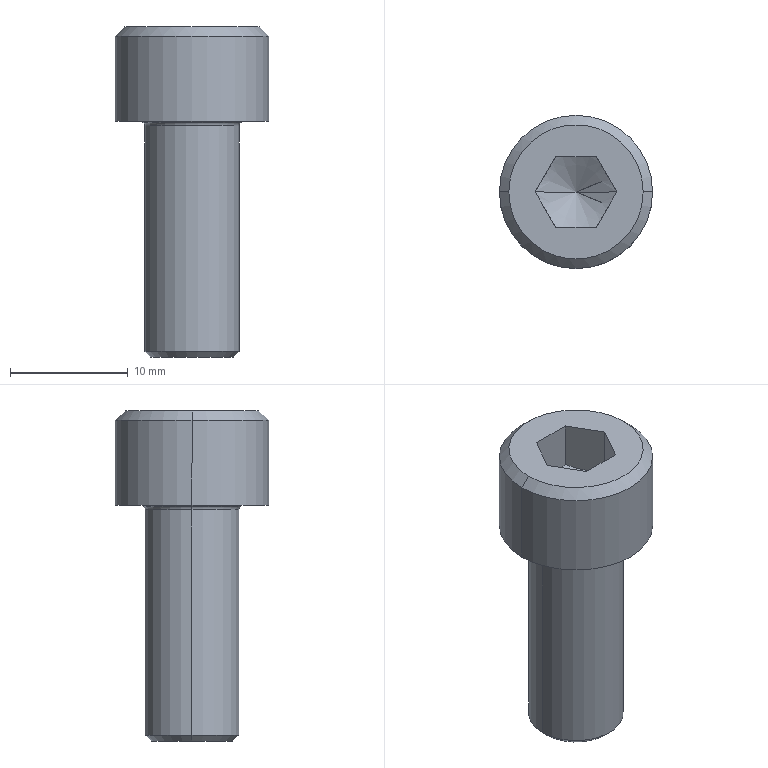Part | Creo | 1 solid | 23 faces | box 13 x 13 x 28 mm | volume 1903 mm3 | plane 9 | cone 6 | cylinder 4 | torus 4 | commonest cylinder face diameters 8 x2 13 x2
STEP:
#1=CARTESIAN_POINT('',(-151.536,-0.004699,-50.5));
#2=VERTEX_POINT('',#1);
#3=CARTESIAN_POINT('',(-153.268,2.995,-50.5));
#4=VERTEX_POINT('',#3);
#5=CARTESIAN_POINT('',(-151.536,-0.004699,-50.5));
#6=CARTESIAN_POINT('',(-151.583,0.07635,-50.527));
#7=CARTESIAN_POINT('',(-151.675,0.236,-50.577));
#8=CARTESIAN_POINT('',(-151.808,0.4663,-50.639));
#9=CARTESIAN_POINT('',(-151.939,0.6927,-50.689));
#10=CARTESIAN_POINT('',(-152.069,0.9189,-50.728));
#11=CARTESIAN_POINT('',(-152.201,1.148,-50.755));
#12=CARTESIAN_POINT('',(-152.335,1.379,-50.769));
#13=CARTESIAN_POINT('',(-152.469,1.612,-50.769));
#14=CARTESIAN_POINT('',(-152.602,1.843,-50.755));
#15=CARTESIAN_POINT('',(-152.735,2.072,-50.728));
#16=CARTESIAN_POINT('',(-152.865,2.298,-50.689));
#17=CARTESIAN_POINT('',(-152.996,2.524,-50.639));
#18=CARTESIAN_POINT('',(-153.129,2.755,-50.577));
#19=CARTESIAN_POINT('',(-153.221,2.914,-50.527));
#20=CARTESIAN_POINT('',(-153.268,2.995,-50.5));
#21=B_SPLINE_CURVE_WITH_KNOTS('',3,(#5,#6,#7,#8,#9,#10,#11,#12,#13,#14,#15,#16,#17,#18,#19,#20),.UNSPECIFIED.,.F.,.F.,(4,1,1,1,1,1,1,1,1,1,1,1,1,4),(0.,0.07692,0.1538,0.2308,0.3077,0.3846,0.4615,0.5385,0.6154,0.6923,0.7692,0.8462,0.9231,1.),.UNSPECIFIED.);
#22=EDGE_CURVE('',#2,#4,#21,.T.);
#23=ORIENTED_EDGE('',*,*,#22,.F.);
#24=CARTESIAN_POINT('',(-155.,-0.004699,-52.5));
#25=VERTEX_POINT('',#24);
#26=CARTESIAN_POINT('',(-155.,-0.004699,-52.5));
#27=DIRECTION('',(0.866,0.,0.5));
#28=VECTOR('',#27,4.);
#29=LINE('',#26,#28);
#30=EDGE_CURVE('',#25,#2,#29,.T.);
#31=ORIENTED_EDGE('',*,*,#30,.F.);
#32=CARTESIAN_POINT('',(-158.464,-0.004699,-50.5));
#33=VERTEX_POINT('',#32);
#34=CARTESIAN_POINT('',(-155.,-0.004699,-52.5));
#35=DIRECTION('',(-0.866,0.,0.5));
#36=VECTOR('',#35,4.);
#37=LINE('',#34,#36);
#38=EDGE_CURVE('',#25,#33,#37,.T.);
#39=ORIENTED_EDGE('',*,*,#38,.T.);
#40=CARTESIAN_POINT('',(-156.732,2.995,-50.5));
#41=VERTEX_POINT('',#40);
#42=CARTESIAN_POINT('',(-156.732,2.995,-50.5));
#43=CARTESIAN_POINT('',(-156.779,2.914,-50.527));
#44=CARTESIAN_POINT('',(-156.871,2.755,-50.577));
#45=CARTESIAN_POINT('',(-157.004,2.524,-50.639));
#46=CARTESIAN_POINT('',(-157.135,2.298,-50.689));
#47=CARTESIAN_POINT('',(-157.265,2.072,-50.728));
#48=CARTESIAN_POINT('',(-157.398,1.843,-50.755));
#49=CARTESIAN_POINT('',(-157.531,1.612,-50.769));
#50=CARTESIAN_POINT('',(-157.665,1.379,-50.769));
#51=CARTESIAN_POINT('',(-157.799,1.148,-50.755));
#52=CARTESIAN_POINT('',(-157.931,0.9189,-50.728));
#53=CARTESIAN_POINT('',(-158.061,0.6927,-50.689));
#54=CARTESIAN_POINT('',(-158.192,0.4663,-50.639));
#55=CARTESIAN_POINT('',(-158.325,0.236,-50.577));
#56=CARTESIAN_POINT('',(-158.417,0.07635,-50.527));
#57=CARTESIAN_POINT('',(-158.464,-0.004699,-50.5));
#58=B_SPLINE_CURVE_WITH_KNOTS('',3,(#42,#43,#44,#45,#46,#47,#48,#49,#50,#51,#52,#53,#54,#55,#56,#57),.UNSPECIFIED.,.F.,.F.,(4,1,1,1,1,1,1,1,1,1,1,1,1,4),(0.,0.07692,0.1538,0.2308,0.3077,0.3846,0.4615,0.5385,0.6154,0.6923,0.7692,0.8462,0.9231,1.),.UNSPECIFIED.);
#59=EDGE_CURVE('',#41,#33,#58,.T.);
#60=ORIENTED_EDGE('',*,*,#59,.F.);
#61=CARTESIAN_POINT('',(-153.268,2.995,-50.5));
#62=CARTESIAN_POINT('',(-153.361,2.995,-50.527));
#63=CARTESIAN_POINT('',(-153.545,2.995,-50.577));
#64=CARTESIAN_POINT('',(-153.811,2.995,-50.639));
#65=CARTESIAN_POINT('',(-154.072,2.995,-50.689));
#66=CARTESIAN_POINT('',(-154.333,2.995,-50.728));
#67=CARTESIAN_POINT('',(-154.598,2.995,-50.755));
#68=CARTESIAN_POINT('',(-154.865,2.995,-50.769));
#69=CARTESIAN_POINT('',(-155.135,2.995,-50.769));
#70=CARTESIAN_POINT('',(-155.402,2.995,-50.755));
#71=CARTESIAN_POINT('',(-155.667,2.995,-50.728));
#72=CARTESIAN_POINT('',(-155.928,2.995,-50.689));
#73=CARTESIAN_POINT('',(-156.189,2.995,-50.639));
#74=CARTESIAN_POINT('',(-156.455,2.995,-50.577));
#75=CARTESIAN_POINT('',(-156.639,2.995,-50.527));
#76=CARTESIAN_POINT('',(-156.732,2.995,-50.5));
#77=B_SPLINE_CURVE_WITH_KNOTS('',3,(#61,#62,#63,#64,#65,#66,#67,#68,#69,#70,#71,#72,#73,#74,#75,#76),.UNSPECIFIED.,.F.,.F.,(4,1,1,1,1,1,1,1,1,1,1,1,1,4),(0.,0.07692,0.1538,0.2308,0.3077,0.3846,0.4615,0.5385,0.6154,0.6923,0.7692,0.8462,0.9231,1.),.UNSPECIFIED.);
#78=EDGE_CURVE('',#4,#41,#77,.T.);
#79=ORIENTED_EDGE('',*,*,#78,.F.);
#80=EDGE_LOOP('',(#23,#31,#39,#60,#79));
#81=FACE_OUTER_BOUND('',#80,.F.);
#82=CARTESIAN_POINT('',(-155.,-0.004699,-51.48));
#83=DIRECTION('',(0.,0.,1.));
#84=DIRECTION('',(1.,0.,0.));
#85=AXIS2_PLACEMENT_3D('',#82,#83,#84);
#86=CONICAL_SURFACE('',#85,1.767,60.);
#87=ADVANCED_FACE('',(#81),#86,.F.);
#88=CARTESIAN_POINT('',(-153.268,2.995,-46.5));
#89=VERTEX_POINT('',#88);
#90=CARTESIAN_POINT('',(-151.536,-0.004699,-46.5));
#91=VERTEX_POINT('',#90);
#92=CARTESIAN_POINT('',(-153.268,2.995,-46.5));
#93=DIRECTION('',(0.5,-0.866,0.));
#94=VECTOR('',#93,3.464);
#95=LINE('',#92,#94);
#96=EDGE_CURVE('',#89,#91,#95,.T.);
#97=ORIENTED_EDGE('',*,*,#96,.T.);
#98=CARTESIAN_POINT('',(-151.536,-0.004699,-46.5));
#99=DIRECTION('',(0.,0.,-1.));
#100=VECTOR('',#99,4.);
#101=LINE('',#98,#100);
#102=EDGE_CURVE('',#91,#2,#101,.T.);
#103=ORIENTED_EDGE('',*,*,#102,.T.);
#104=ORIENTED_EDGE('',*,*,#22,.T.);
#105=CARTESIAN_POINT('',(-153.268,2.995,-46.5));
#106=DIRECTION('',(0.,0.,-1.));
#107=VECTOR('',#106,4.);
#108=LINE('',#105,#107);
#109=EDGE_CURVE('',#89,#4,#108,.T.);
#110=ORIENTED_EDGE('',*,*,#109,.F.);
#111=EDGE_LOOP('',(#97,#103,#104,#110));
#112=FACE_OUTER_BOUND('',#111,.F.);
#113=CARTESIAN_POINT('',(-153.268,2.995,-50.5));
#114=DIRECTION('',(-0.866,-0.5,0.));
#115=DIRECTION('',(0.5,-0.866,0.));
#116=AXIS2_PLACEMENT_3D('',#113,#114,#115);
#117=PLANE('',#116);
#118=ADVANCED_FACE('',(#112),#117,.T.);
#119=CARTESIAN_POINT('',(-149.3,-0.004699,-46.5));
#120=VERTEX_POINT('',#119);
#121=CARTESIAN_POINT('',(-160.7,-0.004699,-46.5));
#122=VERTEX_POINT('',#121);
#123=CARTESIAN_POINT('',(-155.,-0.004699,-46.5));
#124=DIRECTION('',(0.,0.,1.));
#125=DIRECTION('',(1.,0.,0.));
#126=AXIS2_PLACEMENT_3D('',#123,#124,#125);
#127=CIRCLE('',#126,5.7);
#128=EDGE_CURVE('',#120,#122,#127,.T.);
#129=ORIENTED_EDGE('',*,*,#128,.F.);
#130=CARTESIAN_POINT('',(-155.,-0.004699,-46.5));
#131=DIRECTION('',(0.,0.,1.));
#132=DIRECTION('',(-1.,0.,0.));
#133=AXIS2_PLACEMENT_3D('',#130,#131,#132);
#134=CIRCLE('',#133,5.7);
#135=EDGE_CURVE('',#122,#120,#134,.T.);
#136=ORIENTED_EDGE('',*,*,#135,.F.);
#137=EDGE_LOOP('',(#129,#136));
#138=FACE_OUTER_BOUND('',#137,.F.);
#139=CARTESIAN_POINT('',(-153.268,-3.005,-46.5));
#140=VERTEX_POINT('',#139);
#141=CARTESIAN_POINT('',(-151.536,-0.004699,-46.5));
#142=DIRECTION('',(-0.5,-0.866,0.));
#143=VECTOR('',#142,3.464);
#144=LINE('',#141,#143);
#145=EDGE_CURVE('',#91,#140,#144,.T.);
#146=ORIENTED_EDGE('',*,*,#145,.F.);
#147=ORIENTED_EDGE('',*,*,#96,.F.);
#148=CARTESIAN_POINT('',(-156.732,2.995,-46.5));
#149=VERTEX_POINT('',#148);
#150=CARTESIAN_POINT('',(-153.268,2.995,-46.5));
#151=DIRECTION('',(-1.,0.,0.));
#152=VECTOR('',#151,3.464);
#153=LINE('',#150,#152);
#154=EDGE_CURVE('',#89,#149,#153,.T.);
#155=ORIENTED_EDGE('',*,*,#154,.T.);
#156=CARTESIAN_POINT('',(-158.464,-0.004699,-46.5));
#157=VERTEX_POINT('',#156);
#158=CARTESIAN_POINT('',(-158.464,-0.004699,-46.5));
#159=DIRECTION('',(0.5,0.866,0.));
#160=VECTOR('',#159,3.464);
#161=LINE('',#158,#160);
#162=EDGE_CURVE('',#157,#149,#161,.T.);
#163=ORIENTED_EDGE('',*,*,#162,.F.);
#164=CARTESIAN_POINT('',(-156.732,-3.005,-46.5));
#165=VERTEX_POINT('',#164);
#166=CARTESIAN_POINT('',(-156.732,-3.005,-46.5));
#167=DIRECTION('',(-0.5,0.866,0.));
#168=VECTOR('',#167,3.464);
#169=LINE('',#166,#168);
#170=EDGE_CURVE('',#165,#157,#169,.T.);
#171=ORIENTED_EDGE('',*,*,#170,.F.);
#172=CARTESIAN_POINT('',(-156.732,-3.005,-46.5));
#173=DIRECTION('',(1.,0.,0.));
#174=VECTOR('',#173,3.464);
#175=LINE('',#172,#174);
#176=EDGE_CURVE('',#165,#140,#175,.T.);
#177=ORIENTED_EDGE('',*,*,#176,.T.);
#178=EDGE_LOOP('',(#146,#147,#155,#163,#171,#177));
#179=FACE_BOUND('',#178,.F.);
#180=CARTESIAN_POINT('',(-155.,-0.004699,-46.5));
#181=DIRECTION('',(0.,0.,1.));
#182=DIRECTION('',(1.,0.,0.));
#183=AXIS2_PLACEMENT_3D('',#180,#181,#182);
#184=PLANE('',#183);
#185=ADVANCED_FACE('',(#138,#179),#184,.T.);
#186=CARTESIAN_POINT('',(-148.5,-0.004699,-47.3));
#187=VERTEX_POINT('',#186);
#188=CARTESIAN_POINT('',(-161.5,-0.004699,-47.3));
#189=VERTEX_POINT('',#188);
#190=CARTESIAN_POINT('',(-155.,-0.004699,-47.3));
#191=DIRECTION('',(0.,0.,1.));
#192=DIRECTION('',(1.,0.,0.));
#193=AXIS2_PLACEMENT_3D('',#190,#191,#192);
#194=CIRCLE('',#193,6.5);
#195=EDGE_CURVE('',#187,#189,#194,.T.);
#196=ORIENTED_EDGE('',*,*,#195,.F.);
#197=CARTESIAN_POINT('',(-149.3,-0.004699,-46.5));
#198=DIRECTION('',(0.7071,0.,-0.7071));
#199=VECTOR('',#198,1.131);
#200=LINE('',#197,#199);
#201=EDGE_CURVE('',#120,#187,#200,.T.);
#202=ORIENTED_EDGE('',*,*,#201,.F.);
#203=ORIENTED_EDGE('',*,*,#128,.T.);
#204=CARTESIAN_POINT('',(-160.7,-0.004699,-46.5));
#205=DIRECTION('',(-0.7071,0.,-0.7071));
#206=VECTOR('',#205,1.131);
#207=LINE('',#204,#206);
#208=EDGE_CURVE('',#122,#189,#207,.T.);
#209=ORIENTED_EDGE('',*,*,#208,.T.);
#210=EDGE_LOOP('',(#196,#202,#203,#209));
#211=FACE_OUTER_BOUND('',#210,.F.);
#212=CARTESIAN_POINT('',(-155.,-0.004699,-46.9));
#213=DIRECTION('',(0.,0.,-1.));
#214=DIRECTION('',(-1.,0.,0.));
#215=AXIS2_PLACEMENT_3D('',#212,#213,#214);
#216=CONICAL_SURFACE('',#215,6.1,45.);
#217=ADVANCED_FACE('',(#211),#216,.T.);
#218=ORIENTED_EDGE('',*,*,#195,.T.);
#219=CARTESIAN_POINT('',(-161.5,-0.004699,-54.5));
#220=VERTEX_POINT('',#219);
#221=CARTESIAN_POINT('',(-161.5,-0.004699,-54.5));
#222=DIRECTION('',(0.,0.,1.));
#223=VECTOR('',#222,7.2);
#224=LINE('',#221,#223);
#225=EDGE_CURVE('',#220,#189,#224,.T.);
#226=ORIENTED_EDGE('',*,*,#225,.F.);
#227=CARTESIAN_POINT('',(-148.5,-0.004699,-54.5));
#228=VERTEX_POINT('',#227);
#229=CARTESIAN_POINT('',(-155.,-0.004699,-54.5));
#230=DIRECTION('',(0.,0.,-1.));
#231=DIRECTION('',(-1.,0.,0.));
#232=AXIS2_PLACEMENT_3D('',#229,#230,#231);
#233=CIRCLE('',#232,6.5);
#234=EDGE_CURVE('',#220,#228,#233,.T.);
#235=ORIENTED_EDGE('',*,*,#234,.T.);
#236=CARTESIAN_POINT('',(-148.5,-0.004699,-54.5));
#237=DIRECTION('',(0.,0.,1.));
#238=VECTOR('',#237,7.2);
#239=LINE('',#236,#238);
#240=EDGE_CURVE('',#228,#187,#239,.T.);
#241=ORIENTED_EDGE('',*,*,#240,.T.);
#242=EDGE_LOOP('',(#218,#226,#235,#241));
#243=FACE_OUTER_BOUND('',#242,.F.);
#244=CARTESIAN_POINT('',(-155.,-0.004699,-54.5));
#245=DIRECTION('',(0.,0.,1.));
#246=DIRECTION('',(1.,0.,0.));
#247=AXIS2_PLACEMENT_3D('',#244,#245,#246);
#248=CYLINDRICAL_SURFACE('',#247,6.5);
#249=ADVANCED_FACE('',(#243),#248,.T.);
#250=CARTESIAN_POINT('',(-155.,-0.004699,-47.3));
#251=DIRECTION('',(0.,0.,1.));
#252=DIRECTION('',(-1.,0.,0.));
#253=AXIS2_PLACEMENT_3D('',#250,#251,#252);
#254=CIRCLE('',#253,6.5);
#255=EDGE_CURVE('',#189,#187,#254,.T.);
#256=ORIENTED_EDGE('',*,*,#255,.T.);
#257=ORIENTED_EDGE('',*,*,#240,.F.);
#258=CARTESIAN_POINT('',(-155.,-0.004699,-54.5));
#259=DIRECTION('',(0.,0.,-1.));
#260=DIRECTION('',(1.,0.,0.));
#261=AXIS2_PLACEMENT_3D('',#258,#259,#260);
#262=CIRCLE('',#261,6.5);
#263=EDGE_CURVE('',#228,#220,#262,.T.);
#264=ORIENTED_EDGE('',*,*,#263,.T.);
#265=ORIENTED_EDGE('',*,*,#225,.T.);
#266=EDGE_LOOP('',(#256,#257,#264,#265));
#267=FACE_OUTER_BOUND('',#266,.F.);
#268=CARTESIAN_POINT('',(-155.,-0.004699,-54.5));
#269=DIRECTION('',(0.,0.,1.));
#270=DIRECTION('',(1.,0.,0.));
#271=AXIS2_PLACEMENT_3D('',#268,#269,#270);
#272=CYLINDRICAL_SURFACE('',#271,6.5);
#273=ADVANCED_FACE('',(#267),#272,.T.);
#274=ORIENTED_EDGE('',*,*,#255,.F.);
#275=ORIENTED_EDGE('',*,*,#208,.F.);
#276=ORIENTED_EDGE('',*,*,#135,.T.);
#277=ORIENTED_EDGE('',*,*,#201,.T.);
#278=EDGE_LOOP('',(#274,#275,#276,#277));
#279=FACE_OUTER_BOUND('',#278,.F.);
#280=CARTESIAN_POINT('',(-155.,-0.004699,-46.9));
#281=DIRECTION('',(0.,0.,-1.));
#282=DIRECTION('',(-1.,0.,0.));
#283=AXIS2_PLACEMENT_3D('',#280,#281,#282);
#284=CONICAL_SURFACE('',#283,6.1,45.);
#285=ADVANCED_FACE('',(#279),#284,.T.);
#286=ORIENTED_EDGE('',*,*,#263,.F.);
#287=ORIENTED_EDGE('',*,*,#234,.F.);
#288=EDGE_LOOP('',(#286,#287));
#289=FACE_OUTER_BOUND('',#288,.F.);
#290=CARTESIAN_POINT('',(-150.6,-0.004699,-54.5));
#291=VERTEX_POINT('',#290);
#292=CARTESIAN_POINT('',(-159.4,-0.004699,-54.5));
#293=VERTEX_POINT('',#292);
#294=CARTESIAN_POINT('',(-155.,-0.004699,-54.5));
#295=DIRECTION('',(0.,0.,1.));
#296=DIRECTION('',(1.,0.,0.));
#297=AXIS2_PLACEMENT_3D('',#294,#295,#296);
#298=CIRCLE('',#297,4.4);
#299=EDGE_CURVE('',#291,#293,#298,.T.);
#300=ORIENTED_EDGE('',*,*,#299,.F.);
#301=CARTESIAN_POINT('',(-155.,-0.004699,-54.5));
#302=DIRECTION('',(0.,0.,1.));
#303=DIRECTION('',(-1.,0.,0.));
#304=AXIS2_PLACEMENT_3D('',#301,#302,#303);
#305=CIRCLE('',#304,4.4);
#306=EDGE_CURVE('',#293,#291,#305,.T.);
#307=ORIENTED_EDGE('',*,*,#306,.F.);
#308=EDGE_LOOP('',(#300,#307));
#309=FACE_BOUND('',#308,.F.);
#310=CARTESIAN_POINT('',(-155.,-0.004699,-54.5));
#311=DIRECTION('',(0.,0.,1.));
#312=DIRECTION('',(1.,0.,0.));
#313=AXIS2_PLACEMENT_3D('',#310,#311,#312);
#314=PLANE('',#313);
#315=ADVANCED_FACE('',(#289,#309),#314,.F.);
#316=ORIENTED_EDGE('',*,*,#299,.T.);
#317=CARTESIAN_POINT('',(-159.117,-0.004699,-54.617));
#318=VERTEX_POINT('',#317);
#319=CARTESIAN_POINT('',(-159.4,-0.004699,-54.9));
#320=DIRECTION('',(0.,1.,0.));
#321=DIRECTION('',(0.,0.,1.));
#322=AXIS2_PLACEMENT_3D('',#319,#320,#321);
#323=CIRCLE('',#322,0.4);
#324=EDGE_CURVE('',#293,#318,#323,.T.);
#325=ORIENTED_EDGE('',*,*,#324,.T.);
#326=CARTESIAN_POINT('',(-150.883,-0.004699,-54.617));
#327=VERTEX_POINT('',#326);
#328=CARTESIAN_POINT('',(-155.,-0.004699,-54.617));
#329=DIRECTION('',(0.,0.,1.));
#330=DIRECTION('',(1.,0.,0.));
#331=AXIS2_PLACEMENT_3D('',#328,#329,#330);
#332=CIRCLE('',#331,4.117);
#333=EDGE_CURVE('',#327,#318,#332,.T.);
#334=ORIENTED_EDGE('',*,*,#333,.F.);
#335=CARTESIAN_POINT('',(-150.6,-0.004699,-54.9));
#336=DIRECTION('',(0.,-1.,0.));
#337=DIRECTION('',(0.,0.,1.));
#338=AXIS2_PLACEMENT_3D('',#335,#336,#337);
#339=CIRCLE('',#338,0.4);
#340=EDGE_CURVE('',#291,#327,#339,.T.);
#341=ORIENTED_EDGE('',*,*,#340,.F.);
#342=EDGE_LOOP('',(#316,#325,#334,#341));
#343=FACE_OUTER_BOUND('',#342,.F.);
#344=CARTESIAN_POINT('',(-155.,-0.004699,-54.9));
#345=DIRECTION('',(0.,0.,1.));
#346=DIRECTION('',(1.,0.,0.));
#347=AXIS2_PLACEMENT_3D('',#344,#345,#346);
#348=TOROIDAL_SURFACE('',#347,4.4,0.4);
#349=ADVANCED_FACE('',(#343),#348,.F.);
#350=ORIENTED_EDGE('',*,*,#306,.T.);
#351=ORIENTED_EDGE('',*,*,#340,.T.);
#352=CARTESIAN_POINT('',(-155.,-0.004699,-54.617));
#353=DIRECTION('',(0.,0.,1.));
#354=DIRECTION('',(-1.,0.,0.));
#355=AXIS2_PLACEMENT_3D('',#352,#353,#354);
#356=CIRCLE('',#355,4.117);
#357=EDGE_CURVE('',#318,#327,#356,.T.);
#358=ORIENTED_EDGE('',*,*,#357,.F.);
#359=ORIENTED_EDGE('',*,*,#324,.F.);
#360=EDGE_LOOP('',(#350,#351,#358,#359));
#361=FACE_OUTER_BOUND('',#360,.F.);
#362=CARTESIAN_POINT('',(-155.,-0.004699,-54.9));
#363=DIRECTION('',(0.,0.,1.));
#364=DIRECTION('',(1.,0.,0.));
#365=AXIS2_PLACEMENT_3D('',#362,#363,#364);
#366=TOROIDAL_SURFACE('',#365,4.4,0.4);
#367=ADVANCED_FACE('',(#361),#366,.F.);
#368=CARTESIAN_POINT('',(-159.,-0.004699,-54.9));
#369=VERTEX_POINT('',#368);
#370=CARTESIAN_POINT('',(-151.,-0.004699,-54.9));
#371=VERTEX_POINT('',#370);
#372=CARTESIAN_POINT('',(-155.,-0.004699,-54.9));
#373=DIRECTION('',(0.,0.,1.));
#374=DIRECTION('',(-1.,0.,0.));
#375=AXIS2_PLACEMENT_3D('',#372,#373,#374);
#376=CIRCLE('',#375,4.);
#377=EDGE_CURVE('',#369,#371,#376,.T.);
#378=ORIENTED_EDGE('',*,*,#377,.F.);
#379=CARTESIAN_POINT('',(-159.4,-0.004699,-54.9));
#380=DIRECTION('',(0.,1.,0.));
#381=DIRECTION('',(0.7071,0.,0.7071));
#382=AXIS2_PLACEMENT_3D('',#379,#380,#381);
#383=CIRCLE('',#382,0.4);
#384=EDGE_CURVE('',#318,#369,#383,.T.);
#385=ORIENTED_EDGE('',*,*,#384,.F.);
#386=ORIENTED_EDGE('',*,*,#357,.T.);
#387=CARTESIAN_POINT('',(-150.6,-0.004699,-54.9));
#388=DIRECTION('',(0.,-1.,0.));
#389=DIRECTION('',(-0.7071,0.,0.7071));
#390=AXIS2_PLACEMENT_3D('',#387,#388,#389);
#391=CIRCLE('',#390,0.4);
#392=EDGE_CURVE('',#327,#371,#391,.T.);
#393=ORIENTED_EDGE('',*,*,#392,.T.);
#394=EDGE_LOOP('',(#378,#385,#386,#393));
#395=FACE_OUTER_BOUND('',#394,.F.);
#396=CARTESIAN_POINT('',(-155.,-0.004699,-54.9));
#397=DIRECTION('',(0.,0.,1.));
#398=DIRECTION('',(1.,0.,0.));
#399=AXIS2_PLACEMENT_3D('',#396,#397,#398);
#400=TOROIDAL_SURFACE('',#399,4.4,0.4);
#401=ADVANCED_FACE('',(#395),#400,.F.);
#402=CARTESIAN_POINT('',(-151.,-0.004699,-74.));
#403=VERTEX_POINT('',#402);
#404=CARTESIAN_POINT('',(-159.,-0.004699,-74.));
#405=VERTEX_POINT('',#404);
#406=CARTESIAN_POINT('',(-155.,-0.004699,-74.));
#407=DIRECTION('',(0.,0.,-1.));
#408=DIRECTION('',(1.,0.,0.));
#409=AXIS2_PLACEMENT_3D('',#406,#407,#408);
#410=CIRCLE('',#409,4.);
#411=EDGE_CURVE('',#403,#405,#410,.T.);
#412=ORIENTED_EDGE('',*,*,#411,.T.);
#413=CARTESIAN_POINT('',(-159.,-0.004699,-74.));
#414=DIRECTION('',(0.,0.,1.));
#415=VECTOR('',#414,19.1);
#416=LINE('',#413,#415);
#417=EDGE_CURVE('',#405,#369,#416,.T.);
#418=ORIENTED_EDGE('',*,*,#417,.T.);
#419=ORIENTED_EDGE('',*,*,#377,.T.);
#420=CARTESIAN_POINT('',(-151.,-0.004699,-74.));
#421=DIRECTION('',(0.,0.,1.));
#422=VECTOR('',#421,19.1);
#423=LINE('',#420,#422);
#424=EDGE_CURVE('',#403,#371,#423,.T.);
#425=ORIENTED_EDGE('',*,*,#424,.F.);
#426=EDGE_LOOP('',(#412,#418,#419,#425));
#427=FACE_OUTER_BOUND('',#426,.F.);
#428=CARTESIAN_POINT('',(-155.,-0.004699,-74.5));
#429=DIRECTION('',(0.,0.,1.));
#430=DIRECTION('',(1.,0.,0.));
#431=AXIS2_PLACEMENT_3D('',#428,#429,#430);
#432=CYLINDRICAL_SURFACE('',#431,4.);
#433=ADVANCED_FACE('',(#427),#432,.T.);
#434=CARTESIAN_POINT('',(-151.5,-0.004699,-74.5));
#435=VERTEX_POINT('',#434);
#436=CARTESIAN_POINT('',(-158.5,-0.004699,-74.5));
#437=VERTEX_POINT('',#436);
#438=CARTESIAN_POINT('',(-155.,-0.004699,-74.5));
#439=DIRECTION('',(0.,0.,-1.));
#440=DIRECTION('',(1.,0.,0.));
#441=AXIS2_PLACEMENT_3D('',#438,#439,#440);
#442=CIRCLE('',#441,3.5);
#443=EDGE_CURVE('',#435,#437,#442,.T.);
#444=ORIENTED_EDGE('',*,*,#443,.T.);
#445=CARTESIAN_POINT('',(-158.5,-0.004699,-74.5));
#446=DIRECTION('',(-0.7071,0.,0.7071));
#447=VECTOR('',#446,0.7071);
#448=LINE('',#445,#447);
#449=EDGE_CURVE('',#437,#405,#448,.T.);
#450=ORIENTED_EDGE('',*,*,#449,.T.);
#451=ORIENTED_EDGE('',*,*,#411,.F.);
#452=CARTESIAN_POINT('',(-151.5,-0.004699,-74.5));
#453=DIRECTION('',(0.7071,0.,0.7071));
#454=VECTOR('',#453,0.7071);
#455=LINE('',#452,#454);
#456=EDGE_CURVE('',#435,#403,#455,.T.);
#457=ORIENTED_EDGE('',*,*,#456,.F.);
#458=EDGE_LOOP('',(#444,#450,#451,#457));
#459=FACE_OUTER_BOUND('',#458,.F.);
#460=CARTESIAN_POINT('',(-155.,-0.004699,-74.25));
#461=DIRECTION('',(0.,0.,1.));
#462=DIRECTION('',(1.,0.,0.));
#463=AXIS2_PLACEMENT_3D('',#460,#461,#462);
#464=CONICAL_SURFACE('',#463,3.75,45.);
#465=ADVANCED_FACE('',(#459),#464,.T.);
#466=ORIENTED_EDGE('',*,*,#443,.F.);
#467=CARTESIAN_POINT('',(-155.,-0.004699,-74.5));
#468=DIRECTION('',(0.,0.,-1.));
#469=DIRECTION('',(-1.,0.,0.));
#470=AXIS2_PLACEMENT_3D('',#467,#468,#469);
#471=CIRCLE('',#470,3.5);
#472=EDGE_CURVE('',#437,#435,#471,.T.);
#473=ORIENTED_EDGE('',*,*,#472,.F.);
#474=EDGE_LOOP('',(#466,#473));
#475=FACE_OUTER_BOUND('',#474,.F.);
#476=CARTESIAN_POINT('',(-155.,-0.004699,-74.5));
#477=DIRECTION('',(0.,0.,1.));
#478=DIRECTION('',(1.,0.,0.));
#479=AXIS2_PLACEMENT_3D('',#476,#477,#478);
#480=PLANE('',#479);
#481=ADVANCED_FACE('',(#475),#480,.F.);
#482=ORIENTED_EDGE('',*,*,#472,.T.);
#483=ORIENTED_EDGE('',*,*,#456,.T.);
#484=CARTESIAN_POINT('',(-155.,-0.004699,-74.));
#485=DIRECTION('',(0.,0.,-1.));
#486=DIRECTION('',(-1.,0.,0.));
#487=AXIS2_PLACEMENT_3D('',#484,#485,#486);
#488=CIRCLE('',#487,4.);
#489=EDGE_CURVE('',#405,#403,#488,.T.);
#490=ORIENTED_EDGE('',*,*,#489,.F.);
#491=ORIENTED_EDGE('',*,*,#449,.F.);
#492=EDGE_LOOP('',(#482,#483,#490,#491));
#493=FACE_OUTER_BOUND('',#492,.F.);
#494=CARTESIAN_POINT('',(-155.,-0.004699,-74.25));
#495=DIRECTION('',(0.,0.,1.));
#496=DIRECTION('',(1.,0.,0.));
#497=AXIS2_PLACEMENT_3D('',#494,#495,#496);
#498=CONICAL_SURFACE('',#497,3.75,45.);
#499=ADVANCED_FACE('',(#493),#498,.T.);
#500=ORIENTED_EDGE('',*,*,#489,.T.);
#501=ORIENTED_EDGE('',*,*,#424,.T.);
#502=CARTESIAN_POINT('',(-155.,-0.004699,-54.9));
#503=DIRECTION('',(0.,0.,1.));
#504=DIRECTION('',(1.,0.,0.));
#505=AXIS2_PLACEMENT_3D('',#502,#503,#504);
#506=CIRCLE('',#505,4.);
#507=EDGE_CURVE('',#371,#369,#506,.T.);
#508=ORIENTED_EDGE('',*,*,#507,.T.);
#509=ORIENTED_EDGE('',*,*,#417,.F.);
#510=EDGE_LOOP('',(#500,#501,#508,#509));
#511=FACE_OUTER_BOUND('',#510,.F.);
#512=CARTESIAN_POINT('',(-155.,-0.004699,-74.5));
#513=DIRECTION('',(0.,0.,1.));
#514=DIRECTION('',(1.,0.,0.));
#515=AXIS2_PLACEMENT_3D('',#512,#513,#514);
#516=CYLINDRICAL_SURFACE('',#515,4.);
#517=ADVANCED_FACE('',(#511),#516,.T.);
#518=ORIENTED_EDGE('',*,*,#507,.F.);
#519=ORIENTED_EDGE('',*,*,#392,.F.);
#520=ORIENTED_EDGE('',*,*,#333,.T.);
#521=ORIENTED_EDGE('',*,*,#384,.T.);
#522=EDGE_LOOP('',(#518,#519,#520,#521));
#523=FACE_OUTER_BOUND('',#522,.F.);
#524=CARTESIAN_POINT('',(-155.,-0.004699,-54.9));
#525=DIRECTION('',(0.,0.,1.));
#526=DIRECTION('',(1.,0.,0.));
#527=AXIS2_PLACEMENT_3D('',#524,#525,#526);
#528=TOROIDAL_SURFACE('',#527,4.4,0.4);
#529=ADVANCED_FACE('',(#523),#528,.F.);
#530=ORIENTED_EDGE('',*,*,#145,.T.);
#531=CARTESIAN_POINT('',(-153.268,-3.005,-50.5));
#532=VERTEX_POINT('',#531);
#533=CARTESIAN_POINT('',(-153.268,-3.005,-46.5));
#534=DIRECTION('',(0.,0.,-1.));
#535=VECTOR('',#534,4.);
#536=LINE('',#533,#535);
#537=EDGE_CURVE('',#140,#532,#536,.T.);
#538=ORIENTED_EDGE('',*,*,#537,.T.);
#539=CARTESIAN_POINT('',(-153.268,-3.005,-50.5));
#540=CARTESIAN_POINT('',(-153.221,-2.924,-50.527));
#541=CARTESIAN_POINT('',(-153.129,-2.764,-50.577));
#542=CARTESIAN_POINT('',(-152.996,-2.534,-50.639));
#543=CARTESIAN_POINT('',(-152.865,-2.307,-50.689));
#544=CARTESIAN_POINT('',(-152.735,-2.081,-50.728));
#545=CARTESIAN_POINT('',(-152.602,-1.852,-50.755));
#546=CARTESIAN_POINT('',(-152.469,-1.621,-50.769));
#547=CARTESIAN_POINT('',(-152.335,-1.388,-50.769));
#548=CARTESIAN_POINT('',(-152.201,-1.157,-50.755));
#549=CARTESIAN_POINT('',(-152.069,-0.9283,-50.728));
#550=CARTESIAN_POINT('',(-151.939,-0.7021,-50.689));
#551=CARTESIAN_POINT('',(-151.808,-0.4757,-50.639));
#552=CARTESIAN_POINT('',(-151.675,-0.2454,-50.577));
#553=CARTESIAN_POINT('',(-151.583,-0.08575,-50.527));
#554=CARTESIAN_POINT('',(-151.536,-0.004699,-50.5));
#555=B_SPLINE_CURVE_WITH_KNOTS('',3,(#539,#540,#541,#542,#543,#544,#545,#546,#547,#548,#549,#550,#551,#552,#553,#554),.UNSPECIFIED.,.F.,.F.,(4,1,1,1,1,1,1,1,1,1,1,1,1,4),(0.,0.07692,0.1538,0.2308,0.3077,0.3846,0.4615,0.5385,0.6154,0.6923,0.7692,0.8462,0.9231,1.),.UNSPECIFIED.);
#556=EDGE_CURVE('',#532,#2,#555,.T.);
#557=ORIENTED_EDGE('',*,*,#556,.T.);
#558=ORIENTED_EDGE('',*,*,#102,.F.);
#559=EDGE_LOOP('',(#530,#538,#557,#558));
#560=FACE_OUTER_BOUND('',#559,.F.);
#561=CARTESIAN_POINT('',(-151.536,-0.004699,-50.5));
#562=DIRECTION('',(-0.866,0.5,0.));
#563=DIRECTION('',(-0.5,-0.866,0.));
#564=AXIS2_PLACEMENT_3D('',#561,#562,#563);
#565=PLANE('',#564);
#566=ADVANCED_FACE('',(#560),#565,.T.);
#567=ORIENTED_EDGE('',*,*,#176,.F.);
#568=CARTESIAN_POINT('',(-156.732,-3.005,-50.5));
#569=VERTEX_POINT('',#568);
#570=CARTESIAN_POINT('',(-156.732,-3.005,-46.5));
#571=DIRECTION('',(0.,0.,-1.));
#572=VECTOR('',#571,4.);
#573=LINE('',#570,#572);
#574=EDGE_CURVE('',#165,#569,#573,.T.);
#575=ORIENTED_EDGE('',*,*,#574,.T.);
#576=CARTESIAN_POINT('',(-156.732,-3.005,-50.5));
#577=CARTESIAN_POINT('',(-156.639,-3.005,-50.527));
#578=CARTESIAN_POINT('',(-156.455,-3.005,-50.577));
#579=CARTESIAN_POINT('',(-156.189,-3.005,-50.639));
#580=CARTESIAN_POINT('',(-155.928,-3.005,-50.689));
#581=CARTESIAN_POINT('',(-155.667,-3.005,-50.728));
#582=CARTESIAN_POINT('',(-155.402,-3.005,-50.755));
#583=CARTESIAN_POINT('',(-155.135,-3.005,-50.769));
#584=CARTESIAN_POINT('',(-154.865,-3.005,-50.769));
#585=CARTESIAN_POINT('',(-154.598,-3.005,-50.755));
#586=CARTESIAN_POINT('',(-154.333,-3.005,-50.728));
#587=CARTESIAN_POINT('',(-154.072,-3.005,-50.689));
#588=CARTESIAN_POINT('',(-153.811,-3.005,-50.639));
#589=CARTESIAN_POINT('',(-153.545,-3.005,-50.577));
#590=CARTESIAN_POINT('',(-153.361,-3.005,-50.527));
#591=CARTESIAN_POINT('',(-153.268,-3.005,-50.5));
#592=B_SPLINE_CURVE_WITH_KNOTS('',3,(#576,#577,#578,#579,#580,#581,#582,#583,#584,#585,#586,#587,#588,#589,#590,#591),.UNSPECIFIED.,.F.,.F.,(4,1,1,1,1,1,1,1,1,1,1,1,1,4),(0.,0.07692,0.1538,0.2308,0.3077,0.3846,0.4615,0.5385,0.6154,0.6923,0.7692,0.8462,0.9231,1.),.UNSPECIFIED.);
#593=EDGE_CURVE('',#569,#532,#592,.T.);
#594=ORIENTED_EDGE('',*,*,#593,.T.);
#595=ORIENTED_EDGE('',*,*,#537,.F.);
#596=EDGE_LOOP('',(#567,#575,#594,#595));
#597=FACE_OUTER_BOUND('',#596,.F.);
#598=CARTESIAN_POINT('',(-153.268,-3.005,-50.5));
#599=DIRECTION('',(0.,1.,0.));
#600=DIRECTION('',(0.,0.,1.));
#601=AXIS2_PLACEMENT_3D('',#598,#599,#600);
#602=PLANE('',#601);
#603=ADVANCED_FACE('',(#597),#602,.T.);
#604=ORIENTED_EDGE('',*,*,#170,.T.);
#605=CARTESIAN_POINT('',(-158.464,-0.004699,-46.5));
#606=DIRECTION('',(0.,0.,-1.));
#607=VECTOR('',#606,4.);
#608=LINE('',#605,#607);
#609=EDGE_CURVE('',#157,#33,#608,.T.);
#610=ORIENTED_EDGE('',*,*,#609,.T.);
#611=CARTESIAN_POINT('',(-158.464,-0.004699,-50.5));
#612=CARTESIAN_POINT('',(-158.417,-0.08575,-50.527));
#613=CARTESIAN_POINT('',(-158.325,-0.2454,-50.577));
#614=CARTESIAN_POINT('',(-158.192,-0.4757,-50.639));
#615=CARTESIAN_POINT('',(-158.061,-0.7021,-50.689));
#616=CARTESIAN_POINT('',(-157.931,-0.9283,-50.728));
#617=CARTESIAN_POINT('',(-157.799,-1.157,-50.755));
#618=CARTESIAN_POINT('',(-157.665,-1.388,-50.769));
#619=CARTESIAN_POINT('',(-157.531,-1.621,-50.769));
#620=CARTESIAN_POINT('',(-157.398,-1.852,-50.755));
#621=CARTESIAN_POINT('',(-157.265,-2.081,-50.728));
#622=CARTESIAN_POINT('',(-157.135,-2.307,-50.689));
#623=CARTESIAN_POINT('',(-157.004,-2.534,-50.639));
#624=CARTESIAN_POINT('',(-156.871,-2.764,-50.577));
#625=CARTESIAN_POINT('',(-156.779,-2.924,-50.527));
#626=CARTESIAN_POINT('',(-156.732,-3.005,-50.5));
#627=B_SPLINE_CURVE_WITH_KNOTS('',3,(#611,#612,#613,#614,#615,#616,#617,#618,#619,#620,#621,#622,#623,#624,#625,#626),.UNSPECIFIED.,.F.,.F.,(4,1,1,1,1,1,1,1,1,1,1,1,1,4),(0.,0.07692,0.1538,0.2308,0.3077,0.3846,0.4615,0.5385,0.6154,0.6923,0.7692,0.8462,0.9231,1.),.UNSPECIFIED.);
#628=EDGE_CURVE('',#33,#569,#627,.T.);
#629=ORIENTED_EDGE('',*,*,#628,.T.);
#630=ORIENTED_EDGE('',*,*,#574,.F.);
#631=EDGE_LOOP('',(#604,#610,#629,#630));
#632=FACE_OUTER_BOUND('',#631,.F.);
#633=CARTESIAN_POINT('',(-156.732,-3.005,-50.5));
#634=DIRECTION('',(0.866,0.5,0.));
#635=DIRECTION('',(-0.5,0.866,0.));
#636=AXIS2_PLACEMENT_3D('',#633,#634,#635);
#637=PLANE('',#636);
#638=ADVANCED_FACE('',(#632),#637,.T.);
#639=ORIENTED_EDGE('',*,*,#162,.T.);
#640=CARTESIAN_POINT('',(-156.732,2.995,-46.5));
#641=DIRECTION('',(0.,0.,-1.));
#642=VECTOR('',#641,4.);
#643=LINE('',#640,#642);
#644=EDGE_CURVE('',#149,#41,#643,.T.);
#645=ORIENTED_EDGE('',*,*,#644,.T.);
#646=ORIENTED_EDGE('',*,*,#59,.T.);
#647=ORIENTED_EDGE('',*,*,#609,.F.);
#648=EDGE_LOOP('',(#639,#645,#646,#647));
#649=FACE_OUTER_BOUND('',#648,.F.);
#650=CARTESIAN_POINT('',(-158.464,-0.004699,-50.5));
#651=DIRECTION('',(0.866,-0.5,0.));
#652=DIRECTION('',(0.5,0.866,0.));
#653=AXIS2_PLACEMENT_3D('',#650,#651,#652);
#654=PLANE('',#653);
#655=ADVANCED_FACE('',(#649),#654,.T.);
#656=ORIENTED_EDGE('',*,*,#154,.F.);
#657=ORIENTED_EDGE('',*,*,#109,.T.);
#658=ORIENTED_EDGE('',*,*,#78,.T.);
#659=ORIENTED_EDGE('',*,*,#644,.F.);
#660=EDGE_LOOP('',(#656,#657,#658,#659));
#661=FACE_OUTER_BOUND('',#660,.F.);
#662=CARTESIAN_POINT('',(-156.732,2.995,-50.5));
#663=DIRECTION('',(0.,-1.,0.));
#664=DIRECTION('',(0.,0.,-1.));
#665=AXIS2_PLACEMENT_3D('',#662,#663,#664);
#666=PLANE('',#665);
#667=ADVANCED_FACE('',(#661),#666,.T.);
#668=ORIENTED_EDGE('',*,*,#628,.F.);
#669=ORIENTED_EDGE('',*,*,#38,.F.);
#670=ORIENTED_EDGE('',*,*,#30,.T.);
#671=ORIENTED_EDGE('',*,*,#556,.F.);
#672=ORIENTED_EDGE('',*,*,#593,.F.);
#673=EDGE_LOOP('',(#668,#669,#670,#671,#672));
#674=FACE_OUTER_BOUND('',#673,.F.);
#675=CARTESIAN_POINT('',(-155.,-0.004699,-51.48));
#676=DIRECTION('',(0.,0.,1.));
#677=DIRECTION('',(1.,0.,0.));
#678=AXIS2_PLACEMENT_3D('',#675,#676,#677);
#679=CONICAL_SURFACE('',#678,1.767,60.);
#680=ADVANCED_FACE('',(#674),#679,.F.);
#681=CLOSED_SHELL('',(#87,#118,#185,#217,#249,#273,#285,#315,#349,#367,#401,#433,#465,#481,#499,#517,#529,#566,#603,#638,#655,#667,#680));
#682=MANIFOLD_SOLID_BREP('',#681);
#683=(LENGTH_UNIT()NAMED_UNIT(*)SI_UNIT(.MILLI.,.METRE.));
#684=UNCERTAINTY_MEASURE_WITH_UNIT(LENGTH_MEASURE(0.003349),#683,'','');
#685=(NAMED_UNIT(*)PLANE_ANGLE_UNIT()SI_UNIT($,.RADIAN.));
#686=PLANE_ANGLE_MEASURE_WITH_UNIT(PLANE_ANGLE_MEASURE(0.01745),#685);
#687=(CONVERSION_BASED_UNIT('DEGREE',#686)NAMED_UNIT(*)PLANE_ANGLE_UNIT());
#688=(NAMED_UNIT(*)SI_UNIT($,.STERADIAN.)SOLID_ANGLE_UNIT());
#689=(GEOMETRIC_REPRESENTATION_CONTEXT(3)GLOBAL_UNCERTAINTY_ASSIGNED_CONTEXT((#684))GLOBAL_UNIT_ASSIGNED_CONTEXT((#683,#687,#688))REPRESENTATION_CONTEXT('',''));
#690=ADVANCED_BREP_SHAPE_REPRESENTATION('',(#682),#689);